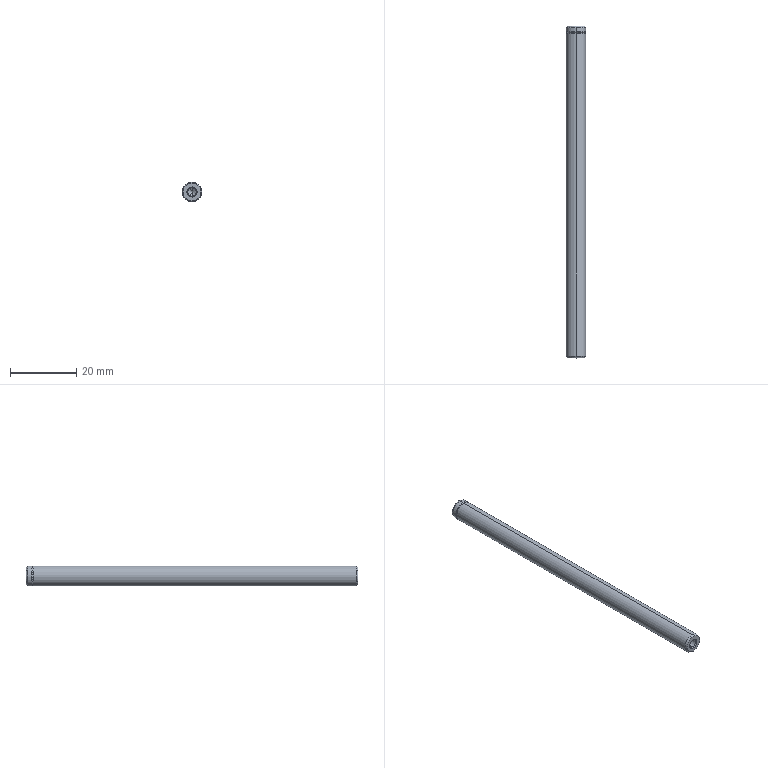Part | STEP file | MOP-100-1.step-7.STEP.STEP-76.STEP | 1 solid | 26 faces | box 6 x 100 x 6 mm | volume 2776 mm3 | cone 16 | cylinder 8 | plane 2 | commonest cylinder face diameters 2.5 x4 6 x4
STEP:
#1=CARTESIAN_POINT('',(0.,97.8,3.));
#2=VERTEX_POINT('',#1);
#3=CARTESIAN_POINT('',(0.,97.8,-3.));
#4=VERTEX_POINT('',#3);
#5=CARTESIAN_POINT('',(0.,97.8,0.));
#6=DIRECTION('',(0.,1.,0.));
#7=DIRECTION('',(0.,0.,-1.));
#8=AXIS2_PLACEMENT_3D('',#5,#6,#7);
#9=CIRCLE('',#8,3.);
#10=EDGE_CURVE('',#2,#4,#9,.T.);
#11=ORIENTED_EDGE('',*,*,#10,.F.);
#12=CARTESIAN_POINT('',(0.,0.5196,3.));
#13=VERTEX_POINT('',#12);
#14=CARTESIAN_POINT('',(0.,100.,3.));
#15=DIRECTION('',(0.,-1.,0.));
#16=VECTOR('',#15,1000.);
#17=LINE('',#14,#16);
#18=EDGE_CURVE('',#2,#13,#17,.T.);
#19=ORIENTED_EDGE('',*,*,#18,.T.);
#20=CARTESIAN_POINT('',(0.,0.5196,-3.));
#21=VERTEX_POINT('',#20);
#22=CARTESIAN_POINT('',(0.,0.5196,0.));
#23=DIRECTION('',(0.,1.,0.));
#24=DIRECTION('',(0.,0.,1.));
#25=AXIS2_PLACEMENT_3D('',#22,#23,#24);
#26=CIRCLE('',#25,3.);
#27=EDGE_CURVE('',#13,#21,#26,.T.);
#28=ORIENTED_EDGE('',*,*,#27,.T.);
#29=CARTESIAN_POINT('',(0.,100.,-3.));
#30=DIRECTION('',(0.,-1.,0.));
#31=VECTOR('',#30,1000.);
#32=LINE('',#29,#31);
#33=EDGE_CURVE('',#4,#21,#32,.T.);
#34=ORIENTED_EDGE('',*,*,#33,.F.);
#35=EDGE_LOOP('',(#11,#19,#28,#34));
#36=FACE_OUTER_BOUND('',#35,.T.);
#37=CARTESIAN_POINT('',(0.,100.,0.));
#38=DIRECTION('',(0.,-1.,0.));
#39=DIRECTION('',(0.,0.,-1.));
#40=AXIS2_PLACEMENT_3D('',#37,#38,#39);
#41=CYLINDRICAL_SURFACE('',#40,3.);
#42=ADVANCED_FACE('',(#36),#41,.T.);
#43=CARTESIAN_POINT('',(0.,0.,-2.7));
#44=VERTEX_POINT('',#43);
#45=CARTESIAN_POINT('',(0.,0.,2.7));
#46=VERTEX_POINT('',#45);
#47=CARTESIAN_POINT('',(0.,0.,0.));
#48=DIRECTION('',(0.,-1.,0.));
#49=DIRECTION('',(0.,0.,1.));
#50=AXIS2_PLACEMENT_3D('',#47,#48,#49);
#51=CIRCLE('',#50,2.7);
#52=EDGE_CURVE('',#44,#46,#51,.T.);
#53=ORIENTED_EDGE('',*,*,#52,.F.);
#54=CARTESIAN_POINT('',(0.,0.5196,-3.));
#55=DIRECTION('',(0.,0.866,-0.5));
#56=VECTOR('',#55,1000.);
#57=LINE('',#54,#56);
#58=EDGE_CURVE('',#44,#21,#57,.T.);
#59=ORIENTED_EDGE('',*,*,#58,.T.);
#60=ORIENTED_EDGE('',*,*,#27,.F.);
#61=CARTESIAN_POINT('',(0.,0.5196,3.));
#62=DIRECTION('',(0.,0.866,0.5));
#63=VECTOR('',#62,1000.);
#64=LINE('',#61,#63);
#65=EDGE_CURVE('',#46,#13,#64,.T.);
#66=ORIENTED_EDGE('',*,*,#65,.F.);
#67=EDGE_LOOP('',(#53,#59,#60,#66));
#68=FACE_OUTER_BOUND('',#67,.T.);
#69=CARTESIAN_POINT('',(0.,0.5196,0.));
#70=DIRECTION('',(0.,1.,0.));
#71=DIRECTION('',(0.,0.,1.));
#72=AXIS2_PLACEMENT_3D('',#69,#70,#71);
#73=CONICAL_SURFACE('',#72,3.,0.5236);
#74=ADVANCED_FACE('',(#68),#73,.T.);
#75=CARTESIAN_POINT('',(0.,0.3,1.25));
#76=VERTEX_POINT('',#75);
#77=CARTESIAN_POINT('',(0.,0.3,-1.25));
#78=VERTEX_POINT('',#77);
#79=CARTESIAN_POINT('',(0.,0.3,0.));
#80=DIRECTION('',(0.,-1.,0.));
#81=DIRECTION('',(0.,0.,1.));
#82=AXIS2_PLACEMENT_3D('',#79,#80,#81);
#83=CIRCLE('',#82,1.25);
#84=EDGE_CURVE('',#76,#78,#83,.T.);
#85=ORIENTED_EDGE('',*,*,#84,.F.);
#86=CARTESIAN_POINT('',(0.,0.,1.55));
#87=VERTEX_POINT('',#86);
#88=CARTESIAN_POINT('',(0.,0.3,1.25));
#89=DIRECTION('',(0.,-0.7071,0.7071));
#90=VECTOR('',#89,1000.);
#91=LINE('',#88,#90);
#92=EDGE_CURVE('',#76,#87,#91,.T.);
#93=ORIENTED_EDGE('',*,*,#92,.T.);
#94=CARTESIAN_POINT('',(0.,0.,-1.55));
#95=VERTEX_POINT('',#94);
#96=CARTESIAN_POINT('',(0.,0.,0.));
#97=DIRECTION('',(0.,1.,0.));
#98=DIRECTION('',(0.,0.,1.));
#99=AXIS2_PLACEMENT_3D('',#96,#97,#98);
#100=CIRCLE('',#99,1.55);
#101=EDGE_CURVE('',#95,#87,#100,.T.);
#102=ORIENTED_EDGE('',*,*,#101,.F.);
#103=CARTESIAN_POINT('',(0.,0.3,-1.25));
#104=DIRECTION('',(0.,-0.7071,-0.7071));
#105=VECTOR('',#104,1000.);
#106=LINE('',#103,#105);
#107=EDGE_CURVE('',#78,#95,#106,.T.);
#108=ORIENTED_EDGE('',*,*,#107,.F.);
#109=EDGE_LOOP('',(#85,#93,#102,#108));
#110=FACE_OUTER_BOUND('',#109,.T.);
#111=CARTESIAN_POINT('',(0.,0.3,0.));
#112=DIRECTION('',(0.,-1.,0.));
#113=DIRECTION('',(0.,0.,-1.));
#114=AXIS2_PLACEMENT_3D('',#111,#112,#113);
#115=CONICAL_SURFACE('',#114,1.25,0.7854);
#116=ADVANCED_FACE('',(#110),#115,.F.);
#117=CARTESIAN_POINT('',(0.,4.5,1.25));
#118=VERTEX_POINT('',#117);
#119=CARTESIAN_POINT('',(0.,4.5,-1.25));
#120=VERTEX_POINT('',#119);
#121=CARTESIAN_POINT('',(0.,4.5,0.));
#122=DIRECTION('',(0.,-1.,0.));
#123=DIRECTION('',(0.,0.,-1.));
#124=AXIS2_PLACEMENT_3D('',#121,#122,#123);
#125=CIRCLE('',#124,1.25);
#126=EDGE_CURVE('',#118,#120,#125,.T.);
#127=ORIENTED_EDGE('',*,*,#126,.F.);
#128=CARTESIAN_POINT('',(0.,0.,1.25));
#129=DIRECTION('',(0.,-1.,0.));
#130=VECTOR('',#129,1000.);
#131=LINE('',#128,#130);
#132=EDGE_CURVE('',#118,#76,#131,.T.);
#133=ORIENTED_EDGE('',*,*,#132,.T.);
#134=ORIENTED_EDGE('',*,*,#84,.T.);
#135=CARTESIAN_POINT('',(0.,0.,-1.25));
#136=DIRECTION('',(0.,-1.,0.));
#137=VECTOR('',#136,1000.);
#138=LINE('',#135,#137);
#139=EDGE_CURVE('',#120,#78,#138,.T.);
#140=ORIENTED_EDGE('',*,*,#139,.F.);
#141=EDGE_LOOP('',(#127,#133,#134,#140));
#142=FACE_OUTER_BOUND('',#141,.T.);
#143=CARTESIAN_POINT('',(0.,0.,0.));
#144=DIRECTION('',(0.,-1.,0.));
#145=DIRECTION('',(0.,0.,-1.));
#146=AXIS2_PLACEMENT_3D('',#143,#144,#145);
#147=CYLINDRICAL_SURFACE('',#146,1.25);
#148=ADVANCED_FACE('',(#142),#147,.F.);
#149=CARTESIAN_POINT('',(0.,5.251,0.));
#150=VERTEX_POINT('',#149);
#151=CARTESIAN_POINT('',(0.,4.5,-1.25));
#152=DIRECTION('',(0.,-0.515,-0.8572));
#153=VECTOR('',#152,1000.);
#154=LINE('',#151,#153);
#155=EDGE_CURVE('',#150,#120,#154,.T.);
#156=ORIENTED_EDGE('',*,*,#155,.F.);
#157=CARTESIAN_POINT('',(0.,4.5,1.25));
#158=DIRECTION('',(0.,-0.515,0.8572));
#159=VECTOR('',#158,1000.);
#160=LINE('',#157,#159);
#161=EDGE_CURVE('',#150,#118,#160,.T.);
#162=ORIENTED_EDGE('',*,*,#161,.T.);
#163=ORIENTED_EDGE('',*,*,#126,.T.);
#164=EDGE_LOOP('',(#156,#162,#163));
#165=FACE_OUTER_BOUND('',#164,.T.);
#166=CARTESIAN_POINT('',(0.,4.5,0.));
#167=DIRECTION('',(0.,-1.,0.));
#168=DIRECTION('',(0.,0.,-1.));
#169=AXIS2_PLACEMENT_3D('',#166,#167,#168);
#170=CONICAL_SURFACE('',#169,1.25,1.03);
#171=ADVANCED_FACE('',(#165),#170,.F.);
#172=CARTESIAN_POINT('',(0.,98.,-2.8));
#173=VERTEX_POINT('',#172);
#174=CARTESIAN_POINT('',(0.,98.,2.8));
#175=VERTEX_POINT('',#174);
#176=CARTESIAN_POINT('',(0.,98.,0.));
#177=DIRECTION('',(0.,-1.,0.));
#178=DIRECTION('',(0.,0.,-1.));
#179=AXIS2_PLACEMENT_3D('',#176,#177,#178);
#180=CIRCLE('',#179,2.8);
#181=EDGE_CURVE('',#173,#175,#180,.T.);
#182=ORIENTED_EDGE('',*,*,#181,.T.);
#183=CARTESIAN_POINT('',(0.,-72.806,173.606));
#184=DIRECTION('',(0.,-0.7071,0.7071));
#185=VECTOR('',#184,1000.);
#186=LINE('',#183,#185);
#187=EDGE_CURVE('',#175,#2,#186,.T.);
#188=ORIENTED_EDGE('',*,*,#187,.T.);
#189=ORIENTED_EDGE('',*,*,#10,.T.);
#190=CARTESIAN_POINT('',(0.,-72.806,-173.606));
#191=DIRECTION('',(0.,-0.7071,-0.7071));
#192=VECTOR('',#191,1000.);
#193=LINE('',#190,#192);
#194=EDGE_CURVE('',#173,#4,#193,.T.);
#195=ORIENTED_EDGE('',*,*,#194,.F.);
#196=EDGE_LOOP('',(#182,#188,#189,#195));
#197=FACE_OUTER_BOUND('',#196,.T.);
#198=CARTESIAN_POINT('',(0.,-72.806,0.));
#199=DIRECTION('',(0.,-1.,0.));
#200=DIRECTION('',(0.,0.,-1.));
#201=AXIS2_PLACEMENT_3D('',#198,#199,#200);
#202=CONICAL_SURFACE('',#201,173.606,0.7854);
#203=ADVANCED_FACE('',(#197),#202,.T.);
#204=ORIENTED_EDGE('',*,*,#181,.F.);
#205=CARTESIAN_POINT('',(0.,98.2,-3.));
#206=VERTEX_POINT('',#205);
#207=CARTESIAN_POINT('',(0.,98.,-2.8));
#208=DIRECTION('',(0.,0.7071,-0.7071));
#209=VECTOR('',#208,1000.);
#210=LINE('',#207,#209);
#211=EDGE_CURVE('',#173,#206,#210,.T.);
#212=ORIENTED_EDGE('',*,*,#211,.T.);
#213=CARTESIAN_POINT('',(0.,98.2,3.));
#214=VERTEX_POINT('',#213);
#215=CARTESIAN_POINT('',(0.,98.2,0.));
#216=DIRECTION('',(0.,-1.,0.));
#217=DIRECTION('',(0.,0.,1.));
#218=AXIS2_PLACEMENT_3D('',#215,#216,#217);
#219=CIRCLE('',#218,3.);
#220=EDGE_CURVE('',#206,#214,#219,.T.);
#221=ORIENTED_EDGE('',*,*,#220,.T.);
#222=CARTESIAN_POINT('',(0.,98.,2.8));
#223=DIRECTION('',(0.,0.7071,0.7071));
#224=VECTOR('',#223,1000.);
#225=LINE('',#222,#224);
#226=EDGE_CURVE('',#175,#214,#225,.T.);
#227=ORIENTED_EDGE('',*,*,#226,.F.);
#228=EDGE_LOOP('',(#204,#212,#221,#227));
#229=FACE_OUTER_BOUND('',#228,.T.);
#230=CARTESIAN_POINT('',(0.,98.,0.));
#231=DIRECTION('',(0.,1.,0.));
#232=DIRECTION('',(0.,0.,1.));
#233=AXIS2_PLACEMENT_3D('',#230,#231,#232);
#234=CONICAL_SURFACE('',#233,2.8,0.7854);
#235=ADVANCED_FACE('',(#229),#234,.T.);
#236=CARTESIAN_POINT('',(0.,99.7,-1.25));
#237=VERTEX_POINT('',#236);
#238=CARTESIAN_POINT('',(0.,99.7,1.25));
#239=VERTEX_POINT('',#238);
#240=CARTESIAN_POINT('',(0.,99.7,0.));
#241=DIRECTION('',(0.,1.,0.));
#242=DIRECTION('',(0.,0.,1.));
#243=AXIS2_PLACEMENT_3D('',#240,#241,#242);
#244=CIRCLE('',#243,1.25);
#245=EDGE_CURVE('',#237,#239,#244,.T.);
#246=ORIENTED_EDGE('',*,*,#245,.F.);
#247=CARTESIAN_POINT('',(0.,100.,-1.55));
#248=VERTEX_POINT('',#247);
#249=CARTESIAN_POINT('',(0.,99.7,-1.25));
#250=DIRECTION('',(0.,0.7071,-0.7071));
#251=VECTOR('',#250,1000.);
#252=LINE('',#249,#251);
#253=EDGE_CURVE('',#237,#248,#252,.T.);
#254=ORIENTED_EDGE('',*,*,#253,.T.);
#255=CARTESIAN_POINT('',(0.,100.,1.55));
#256=VERTEX_POINT('',#255);
#257=CARTESIAN_POINT('',(0.,100.,0.));
#258=DIRECTION('',(0.,-1.,0.));
#259=DIRECTION('',(0.,0.,1.));
#260=AXIS2_PLACEMENT_3D('',#257,#258,#259);
#261=CIRCLE('',#260,1.55);
#262=EDGE_CURVE('',#256,#248,#261,.T.);
#263=ORIENTED_EDGE('',*,*,#262,.F.);
#264=CARTESIAN_POINT('',(0.,99.7,1.25));
#265=DIRECTION('',(0.,0.7071,0.7071));
#266=VECTOR('',#265,1000.);
#267=LINE('',#264,#266);
#268=EDGE_CURVE('',#239,#256,#267,.T.);
#269=ORIENTED_EDGE('',*,*,#268,.F.);
#270=EDGE_LOOP('',(#246,#254,#263,#269));
#271=FACE_OUTER_BOUND('',#270,.T.);
#272=CARTESIAN_POINT('',(0.,99.7,0.));
#273=DIRECTION('',(0.,1.,0.));
#274=DIRECTION('',(0.,0.,1.));
#275=AXIS2_PLACEMENT_3D('',#272,#273,#274);
#276=CONICAL_SURFACE('',#275,1.25,0.7854);
#277=ADVANCED_FACE('',(#271),#276,.F.);
#278=CARTESIAN_POINT('',(0.,100.,2.7));
#279=VERTEX_POINT('',#278);
#280=CARTESIAN_POINT('',(0.,100.,-2.7));
#281=VERTEX_POINT('',#280);
#282=CARTESIAN_POINT('',(0.,100.,0.));
#283=DIRECTION('',(0.,1.,0.));
#284=DIRECTION('',(0.,0.,1.));
#285=AXIS2_PLACEMENT_3D('',#282,#283,#284);
#286=CIRCLE('',#285,2.7);
#287=EDGE_CURVE('',#279,#281,#286,.T.);
#288=ORIENTED_EDGE('',*,*,#287,.F.);
#289=CARTESIAN_POINT('',(0.,99.48,3.));
#290=VERTEX_POINT('',#289);
#291=CARTESIAN_POINT('',(0.,100.,2.7));
#292=DIRECTION('',(0.,-0.866,0.5));
#293=VECTOR('',#292,1000.);
#294=LINE('',#291,#293);
#295=EDGE_CURVE('',#279,#290,#294,.T.);
#296=ORIENTED_EDGE('',*,*,#295,.T.);
#297=CARTESIAN_POINT('',(0.,99.48,-3.));
#298=VERTEX_POINT('',#297);
#299=CARTESIAN_POINT('',(0.,99.48,0.));
#300=DIRECTION('',(0.,-1.,0.));
#301=DIRECTION('',(0.,0.,1.));
#302=AXIS2_PLACEMENT_3D('',#299,#300,#301);
#303=CIRCLE('',#302,3.);
#304=EDGE_CURVE('',#298,#290,#303,.T.);
#305=ORIENTED_EDGE('',*,*,#304,.F.);
#306=CARTESIAN_POINT('',(0.,100.,-2.7));
#307=DIRECTION('',(0.,-0.866,-0.5));
#308=VECTOR('',#307,1000.);
#309=LINE('',#306,#308);
#310=EDGE_CURVE('',#281,#298,#309,.T.);
#311=ORIENTED_EDGE('',*,*,#310,.F.);
#312=EDGE_LOOP('',(#288,#296,#305,#311));
#313=FACE_OUTER_BOUND('',#312,.T.);
#314=CARTESIAN_POINT('',(0.,100.,0.));
#315=DIRECTION('',(0.,-1.,0.));
#316=DIRECTION('',(0.,0.,-1.));
#317=AXIS2_PLACEMENT_3D('',#314,#315,#316);
#318=CONICAL_SURFACE('',#317,2.7,0.5236);
#319=ADVANCED_FACE('',(#313),#318,.T.);
#320=CARTESIAN_POINT('',(0.,95.5,-1.25));
#321=VERTEX_POINT('',#320);
#322=CARTESIAN_POINT('',(0.,95.5,1.25));
#323=VERTEX_POINT('',#322);
#324=CARTESIAN_POINT('',(0.,95.5,0.));
#325=DIRECTION('',(0.,1.,0.));
#326=DIRECTION('',(0.,0.,1.));
#327=AXIS2_PLACEMENT_3D('',#324,#325,#326);
#328=CIRCLE('',#327,1.25);
#329=EDGE_CURVE('',#321,#323,#328,.T.);
#330=ORIENTED_EDGE('',*,*,#329,.F.);
#331=CARTESIAN_POINT('',(0.,100.,-1.25));
#332=DIRECTION('',(0.,1.,0.));
#333=VECTOR('',#332,1000.);
#334=LINE('',#331,#333);
#335=EDGE_CURVE('',#321,#237,#334,.T.);
#336=ORIENTED_EDGE('',*,*,#335,.T.);
#337=ORIENTED_EDGE('',*,*,#245,.T.);
#338=CARTESIAN_POINT('',(0.,100.,1.25));
#339=DIRECTION('',(0.,1.,0.));
#340=VECTOR('',#339,1000.);
#341=LINE('',#338,#340);
#342=EDGE_CURVE('',#323,#239,#341,.T.);
#343=ORIENTED_EDGE('',*,*,#342,.F.);
#344=EDGE_LOOP('',(#330,#336,#337,#343));
#345=FACE_OUTER_BOUND('',#344,.T.);
#346=CARTESIAN_POINT('',(0.,100.,0.));
#347=DIRECTION('',(0.,1.,0.));
#348=DIRECTION('',(0.,0.,1.));
#349=AXIS2_PLACEMENT_3D('',#346,#347,#348);
#350=CYLINDRICAL_SURFACE('',#349,1.25);
#351=ADVANCED_FACE('',(#345),#350,.F.);
#352=CARTESIAN_POINT('',(0.,94.749,0.));
#353=VERTEX_POINT('',#352);
#354=CARTESIAN_POINT('',(0.,95.5,1.25));
#355=DIRECTION('',(0.,0.515,0.8572));
#356=VECTOR('',#355,1000.);
#357=LINE('',#354,#356);
#358=EDGE_CURVE('',#353,#323,#357,.T.);
#359=ORIENTED_EDGE('',*,*,#358,.F.);
#360=CARTESIAN_POINT('',(0.,95.5,-1.25));
#361=DIRECTION('',(0.,0.515,-0.8572));
#362=VECTOR('',#361,1000.);
#363=LINE('',#360,#362);
#364=EDGE_CURVE('',#353,#321,#363,.T.);
#365=ORIENTED_EDGE('',*,*,#364,.T.);
#366=ORIENTED_EDGE('',*,*,#329,.T.);
#367=EDGE_LOOP('',(#359,#365,#366));
#368=FACE_OUTER_BOUND('',#367,.T.);
#369=CARTESIAN_POINT('',(0.,95.5,0.));
#370=DIRECTION('',(0.,1.,0.));
#371=DIRECTION('',(0.,0.,1.));
#372=AXIS2_PLACEMENT_3D('',#369,#370,#371);
#373=CONICAL_SURFACE('',#372,1.25,1.03);
#374=ADVANCED_FACE('',(#368),#373,.F.);
#375=ORIENTED_EDGE('',*,*,#304,.T.);
#376=CARTESIAN_POINT('',(0.,100.,3.));
#377=DIRECTION('',(0.,-1.,0.));
#378=VECTOR('',#377,1000.);
#379=LINE('',#376,#378);
#380=EDGE_CURVE('',#290,#214,#379,.T.);
#381=ORIENTED_EDGE('',*,*,#380,.T.);
#382=ORIENTED_EDGE('',*,*,#220,.F.);
#383=CARTESIAN_POINT('',(0.,100.,-3.));
#384=DIRECTION('',(0.,-1.,0.));
#385=VECTOR('',#384,1000.);
#386=LINE('',#383,#385);
#387=EDGE_CURVE('',#298,#206,#386,.T.);
#388=ORIENTED_EDGE('',*,*,#387,.F.);
#389=EDGE_LOOP('',(#375,#381,#382,#388));
#390=FACE_OUTER_BOUND('',#389,.T.);
#391=CARTESIAN_POINT('',(0.,100.,0.));
#392=DIRECTION('',(0.,-1.,0.));
#393=DIRECTION('',(0.,0.,-1.));
#394=AXIS2_PLACEMENT_3D('',#391,#392,#393);
#395=CYLINDRICAL_SURFACE('',#394,3.);
#396=ADVANCED_FACE('',(#390),#395,.T.);
#397=ORIENTED_EDGE('',*,*,#380,.F.);
#398=CARTESIAN_POINT('',(0.,99.48,0.));
#399=DIRECTION('',(0.,-1.,0.));
#400=DIRECTION('',(0.,0.,1.));
#401=AXIS2_PLACEMENT_3D('',#398,#399,#400);
#402=CIRCLE('',#401,3.);
#403=EDGE_CURVE('',#290,#298,#402,.T.);
#404=ORIENTED_EDGE('',*,*,#403,.T.);
#405=ORIENTED_EDGE('',*,*,#387,.T.);
#406=CARTESIAN_POINT('',(0.,98.2,0.));
#407=DIRECTION('',(0.,-1.,0.));
#408=DIRECTION('',(0.,0.,1.));
#409=AXIS2_PLACEMENT_3D('',#406,#407,#408);
#410=CIRCLE('',#409,3.);
#411=EDGE_CURVE('',#214,#206,#410,.T.);
#412=ORIENTED_EDGE('',*,*,#411,.F.);
#413=EDGE_LOOP('',(#397,#404,#405,#412));
#414=FACE_OUTER_BOUND('',#413,.T.);
#415=CARTESIAN_POINT('',(0.,100.,0.));
#416=DIRECTION('',(0.,-1.,0.));
#417=DIRECTION('',(0.,0.,-1.));
#418=AXIS2_PLACEMENT_3D('',#415,#416,#417);
#419=CYLINDRICAL_SURFACE('',#418,3.);
#420=ADVANCED_FACE('',(#414),#419,.T.);
#421=ORIENTED_EDGE('',*,*,#262,.T.);
#422=CARTESIAN_POINT('',(0.,100.,0.));
#423=DIRECTION('',(0.,-1.,0.));
#424=DIRECTION('',(0.,0.,1.));
#425=AXIS2_PLACEMENT_3D('',#422,#423,#424);
#426=CIRCLE('',#425,1.55);
#427=EDGE_CURVE('',#248,#256,#426,.T.);
#428=ORIENTED_EDGE('',*,*,#427,.T.);
#429=EDGE_LOOP('',(#421,#428));
#430=FACE_BOUND('',#429,.T.);
#431=CARTESIAN_POINT('',(0.,100.,0.));
#432=DIRECTION('',(0.,1.,0.));
#433=DIRECTION('',(0.,0.,1.));
#434=AXIS2_PLACEMENT_3D('',#431,#432,#433);
#435=CIRCLE('',#434,2.7);
#436=EDGE_CURVE('',#281,#279,#435,.T.);
#437=ORIENTED_EDGE('',*,*,#436,.T.);
#438=ORIENTED_EDGE('',*,*,#287,.T.);
#439=EDGE_LOOP('',(#437,#438));
#440=FACE_OUTER_BOUND('',#439,.T.);
#441=CARTESIAN_POINT('',(0.,100.,0.));
#442=DIRECTION('',(0.,1.,0.));
#443=DIRECTION('',(1.,0.,0.));
#444=AXIS2_PLACEMENT_3D('',#441,#442,#443);
#445=PLANE('',#444);
#446=ADVANCED_FACE('',(#430,#440),#445,.T.);
#447=ORIENTED_EDGE('',*,*,#364,.F.);
#448=ORIENTED_EDGE('',*,*,#358,.T.);
#449=CARTESIAN_POINT('',(0.,95.5,0.));
#450=DIRECTION('',(0.,1.,0.));
#451=DIRECTION('',(0.,0.,1.));
#452=AXIS2_PLACEMENT_3D('',#449,#450,#451);
#453=CIRCLE('',#452,1.25);
#454=EDGE_CURVE('',#323,#321,#453,.T.);
#455=ORIENTED_EDGE('',*,*,#454,.T.);
#456=EDGE_LOOP('',(#447,#448,#455));
#457=FACE_OUTER_BOUND('',#456,.T.);
#458=CARTESIAN_POINT('',(0.,95.5,0.));
#459=DIRECTION('',(0.,1.,0.));
#460=DIRECTION('',(0.,0.,1.));
#461=AXIS2_PLACEMENT_3D('',#458,#459,#460);
#462=CONICAL_SURFACE('',#461,1.25,1.03);
#463=ADVANCED_FACE('',(#457),#462,.F.);
#464=ORIENTED_EDGE('',*,*,#335,.F.);
#465=ORIENTED_EDGE('',*,*,#454,.F.);
#466=ORIENTED_EDGE('',*,*,#342,.T.);
#467=CARTESIAN_POINT('',(0.,99.7,0.));
#468=DIRECTION('',(0.,1.,0.));
#469=DIRECTION('',(0.,0.,1.));
#470=AXIS2_PLACEMENT_3D('',#467,#468,#469);
#471=CIRCLE('',#470,1.25);
#472=EDGE_CURVE('',#239,#237,#471,.T.);
#473=ORIENTED_EDGE('',*,*,#472,.T.);
#474=EDGE_LOOP('',(#464,#465,#466,#473));
#475=FACE_OUTER_BOUND('',#474,.T.);
#476=CARTESIAN_POINT('',(0.,100.,0.));
#477=DIRECTION('',(0.,1.,0.));
#478=DIRECTION('',(0.,0.,1.));
#479=AXIS2_PLACEMENT_3D('',#476,#477,#478);
#480=CYLINDRICAL_SURFACE('',#479,1.25);
#481=ADVANCED_FACE('',(#475),#480,.F.);
#482=ORIENTED_EDGE('',*,*,#295,.F.);
#483=ORIENTED_EDGE('',*,*,#436,.F.);
#484=ORIENTED_EDGE('',*,*,#310,.T.);
#485=ORIENTED_EDGE('',*,*,#403,.F.);
#486=EDGE_LOOP('',(#482,#483,#484,#485));
#487=FACE_OUTER_BOUND('',#486,.T.);
#488=CARTESIAN_POINT('',(0.,100.,0.));
#489=DIRECTION('',(0.,-1.,0.));
#490=DIRECTION('',(0.,0.,-1.));
#491=AXIS2_PLACEMENT_3D('',#488,#489,#490);
#492=CONICAL_SURFACE('',#491,2.7,0.5236);
#493=ADVANCED_FACE('',(#487),#492,.T.);
#494=ORIENTED_EDGE('',*,*,#253,.F.);
#495=ORIENTED_EDGE('',*,*,#472,.F.);
#496=ORIENTED_EDGE('',*,*,#268,.T.);
#497=ORIENTED_EDGE('',*,*,#427,.F.);
#498=EDGE_LOOP('',(#494,#495,#496,#497));
#499=FACE_OUTER_BOUND('',#498,.T.);
#500=CARTESIAN_POINT('',(0.,99.7,0.));
#501=DIRECTION('',(0.,1.,0.));
#502=DIRECTION('',(0.,0.,1.));
#503=AXIS2_PLACEMENT_3D('',#500,#501,#502);
#504=CONICAL_SURFACE('',#503,1.25,0.7854);
#505=ADVANCED_FACE('',(#499),#504,.F.);
#506=ORIENTED_EDGE('',*,*,#211,.F.);
#507=CARTESIAN_POINT('',(0.,98.,0.));
#508=DIRECTION('',(0.,-1.,0.));
#509=DIRECTION('',(0.,0.,-1.));
#510=AXIS2_PLACEMENT_3D('',#507,#508,#509);
#511=CIRCLE('',#510,2.8);
#512=EDGE_CURVE('',#175,#173,#511,.T.);
#513=ORIENTED_EDGE('',*,*,#512,.F.);
#514=ORIENTED_EDGE('',*,*,#226,.T.);
#515=ORIENTED_EDGE('',*,*,#411,.T.);
#516=EDGE_LOOP('',(#506,#513,#514,#515));
#517=FACE_OUTER_BOUND('',#516,.T.);
#518=CARTESIAN_POINT('',(0.,98.,0.));
#519=DIRECTION('',(0.,1.,0.));
#520=DIRECTION('',(0.,0.,1.));
#521=AXIS2_PLACEMENT_3D('',#518,#519,#520);
#522=CONICAL_SURFACE('',#521,2.8,0.7854);
#523=ADVANCED_FACE('',(#517),#522,.T.);
#524=ORIENTED_EDGE('',*,*,#187,.F.);
#525=ORIENTED_EDGE('',*,*,#512,.T.);
#526=ORIENTED_EDGE('',*,*,#194,.T.);
#527=CARTESIAN_POINT('',(0.,97.8,0.));
#528=DIRECTION('',(0.,1.,0.));
#529=DIRECTION('',(0.,0.,-1.));
#530=AXIS2_PLACEMENT_3D('',#527,#528,#529);
#531=CIRCLE('',#530,3.);
#532=EDGE_CURVE('',#4,#2,#531,.T.);
#533=ORIENTED_EDGE('',*,*,#532,.T.);
#534=EDGE_LOOP('',(#524,#525,#526,#533));
#535=FACE_OUTER_BOUND('',#534,.T.);
#536=CARTESIAN_POINT('',(0.,-72.806,0.));
#537=DIRECTION('',(0.,-1.,0.));
#538=DIRECTION('',(0.,0.,-1.));
#539=AXIS2_PLACEMENT_3D('',#536,#537,#538);
#540=CONICAL_SURFACE('',#539,173.606,0.7854);
#541=ADVANCED_FACE('',(#535),#540,.T.);
#542=ORIENTED_EDGE('',*,*,#161,.F.);
#543=ORIENTED_EDGE('',*,*,#155,.T.);
#544=CARTESIAN_POINT('',(0.,4.5,0.));
#545=DIRECTION('',(0.,-1.,0.));
#546=DIRECTION('',(0.,0.,-1.));
#547=AXIS2_PLACEMENT_3D('',#544,#545,#546);
#548=CIRCLE('',#547,1.25);
#549=EDGE_CURVE('',#120,#118,#548,.T.);
#550=ORIENTED_EDGE('',*,*,#549,.T.);
#551=EDGE_LOOP('',(#542,#543,#550));
#552=FACE_OUTER_BOUND('',#551,.T.);
#553=CARTESIAN_POINT('',(0.,4.5,0.));
#554=DIRECTION('',(0.,-1.,0.));
#555=DIRECTION('',(0.,0.,-1.));
#556=AXIS2_PLACEMENT_3D('',#553,#554,#555);
#557=CONICAL_SURFACE('',#556,1.25,1.03);
#558=ADVANCED_FACE('',(#552),#557,.F.);
#559=ORIENTED_EDGE('',*,*,#132,.F.);
#560=ORIENTED_EDGE('',*,*,#549,.F.);
#561=ORIENTED_EDGE('',*,*,#139,.T.);
#562=CARTESIAN_POINT('',(0.,0.3,0.));
#563=DIRECTION('',(0.,-1.,0.));
#564=DIRECTION('',(0.,0.,1.));
#565=AXIS2_PLACEMENT_3D('',#562,#563,#564);
#566=CIRCLE('',#565,1.25);
#567=EDGE_CURVE('',#78,#76,#566,.T.);
#568=ORIENTED_EDGE('',*,*,#567,.T.);
#569=EDGE_LOOP('',(#559,#560,#561,#568));
#570=FACE_OUTER_BOUND('',#569,.T.);
#571=CARTESIAN_POINT('',(0.,0.,0.));
#572=DIRECTION('',(0.,-1.,0.));
#573=DIRECTION('',(0.,0.,-1.));
#574=AXIS2_PLACEMENT_3D('',#571,#572,#573);
#575=CYLINDRICAL_SURFACE('',#574,1.25);
#576=ADVANCED_FACE('',(#570),#575,.F.);
#577=ORIENTED_EDGE('',*,*,#92,.F.);
#578=ORIENTED_EDGE('',*,*,#567,.F.);
#579=ORIENTED_EDGE('',*,*,#107,.T.);
#580=CARTESIAN_POINT('',(0.,0.,0.));
#581=DIRECTION('',(0.,1.,0.));
#582=DIRECTION('',(0.,0.,1.));
#583=AXIS2_PLACEMENT_3D('',#580,#581,#582);
#584=CIRCLE('',#583,1.55);
#585=EDGE_CURVE('',#87,#95,#584,.T.);
#586=ORIENTED_EDGE('',*,*,#585,.F.);
#587=EDGE_LOOP('',(#577,#578,#579,#586));
#588=FACE_OUTER_BOUND('',#587,.T.);
#589=CARTESIAN_POINT('',(0.,0.3,0.));
#590=DIRECTION('',(0.,-1.,0.));
#591=DIRECTION('',(0.,0.,-1.));
#592=AXIS2_PLACEMENT_3D('',#589,#590,#591);
#593=CONICAL_SURFACE('',#592,1.25,0.7854);
#594=ADVANCED_FACE('',(#588),#593,.F.);
#595=ORIENTED_EDGE('',*,*,#101,.T.);
#596=ORIENTED_EDGE('',*,*,#585,.T.);
#597=EDGE_LOOP('',(#595,#596));
#598=FACE_BOUND('',#597,.T.);
#599=CARTESIAN_POINT('',(0.,0.,0.));
#600=DIRECTION('',(0.,-1.,0.));
#601=DIRECTION('',(0.,0.,1.));
#602=AXIS2_PLACEMENT_3D('',#599,#600,#601);
#603=CIRCLE('',#602,2.7);
#604=EDGE_CURVE('',#46,#44,#603,.T.);
#605=ORIENTED_EDGE('',*,*,#604,.T.);
#606=ORIENTED_EDGE('',*,*,#52,.T.);
#607=EDGE_LOOP('',(#605,#606));
#608=FACE_OUTER_BOUND('',#607,.T.);
#609=CARTESIAN_POINT('',(0.,0.,0.));
#610=DIRECTION('',(0.,1.,0.));
#611=DIRECTION('',(1.,0.,0.));
#612=AXIS2_PLACEMENT_3D('',#609,#610,#611);
#613=PLANE('',#612);
#614=ADVANCED_FACE('',(#598,#608),#613,.F.);
#615=ORIENTED_EDGE('',*,*,#58,.F.);
#616=ORIENTED_EDGE('',*,*,#604,.F.);
#617=ORIENTED_EDGE('',*,*,#65,.T.);
#618=CARTESIAN_POINT('',(0.,0.5196,0.));
#619=DIRECTION('',(0.,1.,0.));
#620=DIRECTION('',(0.,0.,1.));
#621=AXIS2_PLACEMENT_3D('',#618,#619,#620);
#622=CIRCLE('',#621,3.);
#623=EDGE_CURVE('',#21,#13,#622,.T.);
#624=ORIENTED_EDGE('',*,*,#623,.F.);
#625=EDGE_LOOP('',(#615,#616,#617,#624));
#626=FACE_OUTER_BOUND('',#625,.T.);
#627=CARTESIAN_POINT('',(0.,0.5196,0.));
#628=DIRECTION('',(0.,1.,0.));
#629=DIRECTION('',(0.,0.,1.));
#630=AXIS2_PLACEMENT_3D('',#627,#628,#629);
#631=CONICAL_SURFACE('',#630,3.,0.5236);
#632=ADVANCED_FACE('',(#626),#631,.T.);
#633=ORIENTED_EDGE('',*,*,#18,.F.);
#634=ORIENTED_EDGE('',*,*,#532,.F.);
#635=ORIENTED_EDGE('',*,*,#33,.T.);
#636=ORIENTED_EDGE('',*,*,#623,.T.);
#637=EDGE_LOOP('',(#633,#634,#635,#636));
#638=FACE_OUTER_BOUND('',#637,.T.);
#639=CARTESIAN_POINT('',(0.,100.,0.));
#640=DIRECTION('',(0.,-1.,0.));
#641=DIRECTION('',(0.,0.,-1.));
#642=AXIS2_PLACEMENT_3D('',#639,#640,#641);
#643=CYLINDRICAL_SURFACE('',#642,3.);
#644=ADVANCED_FACE('',(#638),#643,.T.);
#645=CLOSED_SHELL('',(#42,#74,#116,#148,#171,#203,#235,#277,#319,#351,#374,#396,#420,#446,#463,#481,#493,#505,#523,#541,#558,#576,#594,#614,#632,#644));
#646=MANIFOLD_SOLID_BREP('',#645);
#647=CARTESIAN_POINT('',(0.,0.,0.));
#648=DIRECTION('',(0.,0.,1.));
#649=DIRECTION('',(1.,0.,0.));
#650=AXIS2_PLACEMENT_3D('',#647,#648,#649);
#651=(LENGTH_UNIT()NAMED_UNIT(*)SI_UNIT(.MILLI.,.METRE.));
#652=UNCERTAINTY_MEASURE_WITH_UNIT(LENGTH_MEASURE(0.00001),#651,'','');
#653=(NAMED_UNIT(*)PLANE_ANGLE_UNIT()SI_UNIT($,.RADIAN.));
#654=(NAMED_UNIT(*)SI_UNIT($,.STERADIAN.)SOLID_ANGLE_UNIT());
#655=(GEOMETRIC_REPRESENTATION_CONTEXT(3)GLOBAL_UNCERTAINTY_ASSIGNED_CONTEXT((#652))GLOBAL_UNIT_ASSIGNED_CONTEXT((#651,#653,#654))REPRESENTATION_CONTEXT('',''));
#656=ADVANCED_BREP_SHAPE_REPRESENTATION('',(#646,#650),#655);